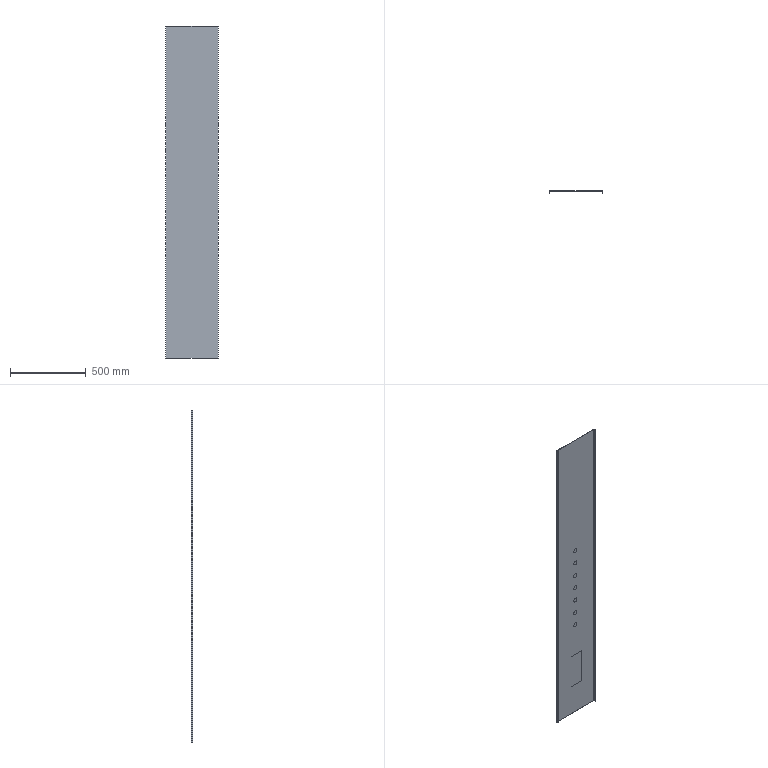Part | SolidWorks | features FlatPattern 1, ICE 1, SMBaseFlange 1, SheetMetal 1 | 1 solid | 48 faces | box 350 x 12 x 2194 mm | volume 1602003 mm3 | plane 30 | cylinder 18 | commonest cylinder face diameters 30 x14 0.4 x2 4.4 x2
STEP:
#1=CARTESIAN_POINT('',(0.,-0.5,685.));
#2=VERTEX_POINT('',#1);
#3=CARTESIAN_POINT('',(0.,-0.5,715.));
#4=VERTEX_POINT('',#3);
#5=CARTESIAN_POINT('',(0.,-0.5,700.));
#6=DIRECTION('',(0.,1.,0.));
#7=DIRECTION('',(0.,0.,1.));
#8=AXIS2_PLACEMENT_3D('',#5,#6,#7);
#9=CIRCLE('',#8,15.);
#10=EDGE_CURVE('',#2,#4,#9,.T.);
#11=ORIENTED_EDGE('',*,*,#10,.F.);
#12=CARTESIAN_POINT('',(0.,0.,685.));
#13=VERTEX_POINT('',#12);
#14=CARTESIAN_POINT('',(0.,-0.5,685.));
#15=DIRECTION('',(0.,1.,0.));
#16=VECTOR('',#15,1000.);
#17=LINE('',#14,#16);
#18=EDGE_CURVE('',#2,#13,#17,.T.);
#19=ORIENTED_EDGE('',*,*,#18,.T.);
#20=CARTESIAN_POINT('',(0.,0.,715.));
#21=VERTEX_POINT('',#20);
#22=CARTESIAN_POINT('',(0.,0.,700.));
#23=DIRECTION('',(0.,1.,0.));
#24=DIRECTION('',(0.,0.,1.));
#25=AXIS2_PLACEMENT_3D('',#22,#23,#24);
#26=CIRCLE('',#25,15.);
#27=EDGE_CURVE('',#13,#21,#26,.T.);
#28=ORIENTED_EDGE('',*,*,#27,.T.);
#29=CARTESIAN_POINT('',(0.,-0.5,715.));
#30=DIRECTION('',(0.,1.,0.));
#31=VECTOR('',#30,1000.);
#32=LINE('',#29,#31);
#33=EDGE_CURVE('',#4,#21,#32,.T.);
#34=ORIENTED_EDGE('',*,*,#33,.F.);
#35=EDGE_LOOP('',(#11,#19,#28,#34));
#36=FACE_OUTER_BOUND('',#35,.T.);
#37=CARTESIAN_POINT('',(0.,-0.5,700.));
#38=DIRECTION('',(0.,1.,0.));
#39=DIRECTION('',(0.,0.,1.));
#40=AXIS2_PLACEMENT_3D('',#37,#38,#39);
#41=CYLINDRICAL_SURFACE('',#40,15.);
#42=ADVANCED_FACE('',(#36),#41,.F.);
#43=CARTESIAN_POINT('',(0.,-0.5,785.));
#44=VERTEX_POINT('',#43);
#45=CARTESIAN_POINT('',(0.,-0.5,815.));
#46=VERTEX_POINT('',#45);
#47=CARTESIAN_POINT('',(0.,-0.5,800.));
#48=DIRECTION('',(0.,1.,0.));
#49=DIRECTION('',(0.,0.,1.));
#50=AXIS2_PLACEMENT_3D('',#47,#48,#49);
#51=CIRCLE('',#50,15.);
#52=EDGE_CURVE('',#44,#46,#51,.T.);
#53=ORIENTED_EDGE('',*,*,#52,.F.);
#54=CARTESIAN_POINT('',(0.,0.,785.));
#55=VERTEX_POINT('',#54);
#56=CARTESIAN_POINT('',(0.,-0.5,785.));
#57=DIRECTION('',(0.,1.,0.));
#58=VECTOR('',#57,1000.);
#59=LINE('',#56,#58);
#60=EDGE_CURVE('',#44,#55,#59,.T.);
#61=ORIENTED_EDGE('',*,*,#60,.T.);
#62=CARTESIAN_POINT('',(0.,0.,815.));
#63=VERTEX_POINT('',#62);
#64=CARTESIAN_POINT('',(0.,0.,800.));
#65=DIRECTION('',(0.,1.,0.));
#66=DIRECTION('',(0.,0.,1.));
#67=AXIS2_PLACEMENT_3D('',#64,#65,#66);
#68=CIRCLE('',#67,15.);
#69=EDGE_CURVE('',#55,#63,#68,.T.);
#70=ORIENTED_EDGE('',*,*,#69,.T.);
#71=CARTESIAN_POINT('',(0.,-0.5,815.));
#72=DIRECTION('',(0.,1.,0.));
#73=VECTOR('',#72,1000.);
#74=LINE('',#71,#73);
#75=EDGE_CURVE('',#46,#63,#74,.T.);
#76=ORIENTED_EDGE('',*,*,#75,.F.);
#77=EDGE_LOOP('',(#53,#61,#70,#76));
#78=FACE_OUTER_BOUND('',#77,.T.);
#79=CARTESIAN_POINT('',(0.,-0.5,800.));
#80=DIRECTION('',(0.,1.,0.));
#81=DIRECTION('',(0.,0.,1.));
#82=AXIS2_PLACEMENT_3D('',#79,#80,#81);
#83=CYLINDRICAL_SURFACE('',#82,15.);
#84=ADVANCED_FACE('',(#78),#83,.F.);
#85=CARTESIAN_POINT('',(0.,-0.5,885.));
#86=VERTEX_POINT('',#85);
#87=CARTESIAN_POINT('',(0.,-0.5,915.));
#88=VERTEX_POINT('',#87);
#89=CARTESIAN_POINT('',(0.,-0.5,900.));
#90=DIRECTION('',(0.,1.,0.));
#91=DIRECTION('',(0.,0.,1.));
#92=AXIS2_PLACEMENT_3D('',#89,#90,#91);
#93=CIRCLE('',#92,15.);
#94=EDGE_CURVE('',#86,#88,#93,.T.);
#95=ORIENTED_EDGE('',*,*,#94,.F.);
#96=CARTESIAN_POINT('',(0.,0.,885.));
#97=VERTEX_POINT('',#96);
#98=CARTESIAN_POINT('',(0.,-0.5,885.));
#99=DIRECTION('',(0.,1.,0.));
#100=VECTOR('',#99,1000.);
#101=LINE('',#98,#100);
#102=EDGE_CURVE('',#86,#97,#101,.T.);
#103=ORIENTED_EDGE('',*,*,#102,.T.);
#104=CARTESIAN_POINT('',(0.,0.,915.));
#105=VERTEX_POINT('',#104);
#106=CARTESIAN_POINT('',(0.,0.,900.));
#107=DIRECTION('',(0.,1.,0.));
#108=DIRECTION('',(0.,0.,1.));
#109=AXIS2_PLACEMENT_3D('',#106,#107,#108);
#110=CIRCLE('',#109,15.);
#111=EDGE_CURVE('',#97,#105,#110,.T.);
#112=ORIENTED_EDGE('',*,*,#111,.T.);
#113=CARTESIAN_POINT('',(0.,-0.5,915.));
#114=DIRECTION('',(0.,1.,0.));
#115=VECTOR('',#114,1000.);
#116=LINE('',#113,#115);
#117=EDGE_CURVE('',#88,#105,#116,.T.);
#118=ORIENTED_EDGE('',*,*,#117,.F.);
#119=EDGE_LOOP('',(#95,#103,#112,#118));
#120=FACE_OUTER_BOUND('',#119,.T.);
#121=CARTESIAN_POINT('',(0.,-0.5,900.));
#122=DIRECTION('',(0.,1.,0.));
#123=DIRECTION('',(0.,0.,1.));
#124=AXIS2_PLACEMENT_3D('',#121,#122,#123);
#125=CYLINDRICAL_SURFACE('',#124,15.);
#126=ADVANCED_FACE('',(#120),#125,.F.);
#127=CARTESIAN_POINT('',(0.,-0.5,985.));
#128=VERTEX_POINT('',#127);
#129=CARTESIAN_POINT('',(0.,-0.5,1015.));
#130=VERTEX_POINT('',#129);
#131=CARTESIAN_POINT('',(0.,-0.5,1000.));
#132=DIRECTION('',(0.,1.,0.));
#133=DIRECTION('',(0.,0.,1.));
#134=AXIS2_PLACEMENT_3D('',#131,#132,#133);
#135=CIRCLE('',#134,15.);
#136=EDGE_CURVE('',#128,#130,#135,.T.);
#137=ORIENTED_EDGE('',*,*,#136,.F.);
#138=CARTESIAN_POINT('',(0.,0.,985.));
#139=VERTEX_POINT('',#138);
#140=CARTESIAN_POINT('',(0.,-0.5,985.));
#141=DIRECTION('',(0.,1.,0.));
#142=VECTOR('',#141,1000.);
#143=LINE('',#140,#142);
#144=EDGE_CURVE('',#128,#139,#143,.T.);
#145=ORIENTED_EDGE('',*,*,#144,.T.);
#146=CARTESIAN_POINT('',(0.,0.,1015.));
#147=VERTEX_POINT('',#146);
#148=CARTESIAN_POINT('',(0.,0.,1000.));
#149=DIRECTION('',(0.,1.,0.));
#150=DIRECTION('',(0.,0.,1.));
#151=AXIS2_PLACEMENT_3D('',#148,#149,#150);
#152=CIRCLE('',#151,15.);
#153=EDGE_CURVE('',#139,#147,#152,.T.);
#154=ORIENTED_EDGE('',*,*,#153,.T.);
#155=CARTESIAN_POINT('',(0.,-0.5,1015.));
#156=DIRECTION('',(0.,1.,0.));
#157=VECTOR('',#156,1000.);
#158=LINE('',#155,#157);
#159=EDGE_CURVE('',#130,#147,#158,.T.);
#160=ORIENTED_EDGE('',*,*,#159,.F.);
#161=EDGE_LOOP('',(#137,#145,#154,#160));
#162=FACE_OUTER_BOUND('',#161,.T.);
#163=CARTESIAN_POINT('',(0.,-0.5,1000.));
#164=DIRECTION('',(0.,1.,0.));
#165=DIRECTION('',(0.,0.,1.));
#166=AXIS2_PLACEMENT_3D('',#163,#164,#165);
#167=CYLINDRICAL_SURFACE('',#166,15.);
#168=ADVANCED_FACE('',(#162),#167,.F.);
#169=CARTESIAN_POINT('',(0.,-0.5,1085.));
#170=VERTEX_POINT('',#169);
#171=CARTESIAN_POINT('',(0.,-0.5,1115.));
#172=VERTEX_POINT('',#171);
#173=CARTESIAN_POINT('',(0.,-0.5,1100.));
#174=DIRECTION('',(0.,1.,0.));
#175=DIRECTION('',(0.,0.,1.));
#176=AXIS2_PLACEMENT_3D('',#173,#174,#175);
#177=CIRCLE('',#176,15.);
#178=EDGE_CURVE('',#170,#172,#177,.T.);
#179=ORIENTED_EDGE('',*,*,#178,.F.);
#180=CARTESIAN_POINT('',(0.,0.,1085.));
#181=VERTEX_POINT('',#180);
#182=CARTESIAN_POINT('',(0.,-0.5,1085.));
#183=DIRECTION('',(0.,1.,0.));
#184=VECTOR('',#183,1000.);
#185=LINE('',#182,#184);
#186=EDGE_CURVE('',#170,#181,#185,.T.);
#187=ORIENTED_EDGE('',*,*,#186,.T.);
#188=CARTESIAN_POINT('',(0.,0.,1115.));
#189=VERTEX_POINT('',#188);
#190=CARTESIAN_POINT('',(0.,0.,1100.));
#191=DIRECTION('',(0.,1.,0.));
#192=DIRECTION('',(0.,0.,1.));
#193=AXIS2_PLACEMENT_3D('',#190,#191,#192);
#194=CIRCLE('',#193,15.);
#195=EDGE_CURVE('',#181,#189,#194,.T.);
#196=ORIENTED_EDGE('',*,*,#195,.T.);
#197=CARTESIAN_POINT('',(0.,-0.5,1115.));
#198=DIRECTION('',(0.,1.,0.));
#199=VECTOR('',#198,1000.);
#200=LINE('',#197,#199);
#201=EDGE_CURVE('',#172,#189,#200,.T.);
#202=ORIENTED_EDGE('',*,*,#201,.F.);
#203=EDGE_LOOP('',(#179,#187,#196,#202));
#204=FACE_OUTER_BOUND('',#203,.T.);
#205=CARTESIAN_POINT('',(0.,-0.5,1100.));
#206=DIRECTION('',(0.,1.,0.));
#207=DIRECTION('',(0.,0.,1.));
#208=AXIS2_PLACEMENT_3D('',#205,#206,#207);
#209=CYLINDRICAL_SURFACE('',#208,15.);
#210=ADVANCED_FACE('',(#204),#209,.F.);
#211=CARTESIAN_POINT('',(0.,-0.5,1185.));
#212=VERTEX_POINT('',#211);
#213=CARTESIAN_POINT('',(0.,-0.5,1215.));
#214=VERTEX_POINT('',#213);
#215=CARTESIAN_POINT('',(0.,-0.5,1200.));
#216=DIRECTION('',(0.,1.,0.));
#217=DIRECTION('',(0.,0.,1.));
#218=AXIS2_PLACEMENT_3D('',#215,#216,#217);
#219=CIRCLE('',#218,15.);
#220=EDGE_CURVE('',#212,#214,#219,.T.);
#221=ORIENTED_EDGE('',*,*,#220,.F.);
#222=CARTESIAN_POINT('',(0.,0.,1185.));
#223=VERTEX_POINT('',#222);
#224=CARTESIAN_POINT('',(0.,-0.5,1185.));
#225=DIRECTION('',(0.,1.,0.));
#226=VECTOR('',#225,1000.);
#227=LINE('',#224,#226);
#228=EDGE_CURVE('',#212,#223,#227,.T.);
#229=ORIENTED_EDGE('',*,*,#228,.T.);
#230=CARTESIAN_POINT('',(0.,0.,1215.));
#231=VERTEX_POINT('',#230);
#232=CARTESIAN_POINT('',(0.,0.,1200.));
#233=DIRECTION('',(0.,1.,0.));
#234=DIRECTION('',(0.,0.,1.));
#235=AXIS2_PLACEMENT_3D('',#232,#233,#234);
#236=CIRCLE('',#235,15.);
#237=EDGE_CURVE('',#223,#231,#236,.T.);
#238=ORIENTED_EDGE('',*,*,#237,.T.);
#239=CARTESIAN_POINT('',(0.,-0.5,1215.));
#240=DIRECTION('',(0.,1.,0.));
#241=VECTOR('',#240,1000.);
#242=LINE('',#239,#241);
#243=EDGE_CURVE('',#214,#231,#242,.T.);
#244=ORIENTED_EDGE('',*,*,#243,.F.);
#245=EDGE_LOOP('',(#221,#229,#238,#244));
#246=FACE_OUTER_BOUND('',#245,.T.);
#247=CARTESIAN_POINT('',(0.,-0.5,1200.));
#248=DIRECTION('',(0.,1.,0.));
#249=DIRECTION('',(0.,0.,1.));
#250=AXIS2_PLACEMENT_3D('',#247,#248,#249);
#251=CYLINDRICAL_SURFACE('',#250,15.);
#252=ADVANCED_FACE('',(#246),#251,.F.);
#253=CARTESIAN_POINT('',(0.,-0.5,1285.));
#254=VERTEX_POINT('',#253);
#255=CARTESIAN_POINT('',(0.,-0.5,1315.));
#256=VERTEX_POINT('',#255);
#257=CARTESIAN_POINT('',(0.,-0.5,1300.));
#258=DIRECTION('',(0.,1.,0.));
#259=DIRECTION('',(0.,0.,1.));
#260=AXIS2_PLACEMENT_3D('',#257,#258,#259);
#261=CIRCLE('',#260,15.);
#262=EDGE_CURVE('',#254,#256,#261,.T.);
#263=ORIENTED_EDGE('',*,*,#262,.F.);
#264=CARTESIAN_POINT('',(0.,0.,1285.));
#265=VERTEX_POINT('',#264);
#266=CARTESIAN_POINT('',(0.,-0.5,1285.));
#267=DIRECTION('',(0.,1.,0.));
#268=VECTOR('',#267,1000.);
#269=LINE('',#266,#268);
#270=EDGE_CURVE('',#254,#265,#269,.T.);
#271=ORIENTED_EDGE('',*,*,#270,.T.);
#272=CARTESIAN_POINT('',(0.,0.,1315.));
#273=VERTEX_POINT('',#272);
#274=CARTESIAN_POINT('',(0.,0.,1300.));
#275=DIRECTION('',(0.,1.,0.));
#276=DIRECTION('',(0.,0.,1.));
#277=AXIS2_PLACEMENT_3D('',#274,#275,#276);
#278=CIRCLE('',#277,15.);
#279=EDGE_CURVE('',#265,#273,#278,.T.);
#280=ORIENTED_EDGE('',*,*,#279,.T.);
#281=CARTESIAN_POINT('',(0.,-0.5,1315.));
#282=DIRECTION('',(0.,1.,0.));
#283=VECTOR('',#282,1000.);
#284=LINE('',#281,#283);
#285=EDGE_CURVE('',#256,#273,#284,.T.);
#286=ORIENTED_EDGE('',*,*,#285,.F.);
#287=EDGE_LOOP('',(#263,#271,#280,#286));
#288=FACE_OUTER_BOUND('',#287,.T.);
#289=CARTESIAN_POINT('',(0.,-0.5,1300.));
#290=DIRECTION('',(0.,1.,0.));
#291=DIRECTION('',(0.,0.,1.));
#292=AXIS2_PLACEMENT_3D('',#289,#290,#291);
#293=CYLINDRICAL_SURFACE('',#292,15.);
#294=ADVANCED_FACE('',(#288),#293,.F.);
#295=CARTESIAN_POINT('',(-172.8,0.,2194.));
#296=VERTEX_POINT('',#295);
#297=CARTESIAN_POINT('',(-172.8,-2.,2194.));
#298=VERTEX_POINT('',#297);
#299=CARTESIAN_POINT('',(-172.8,0.,2194.));
#300=DIRECTION('',(0.,-1.,0.));
#301=VECTOR('',#300,1000.);
#302=LINE('',#299,#301);
#303=EDGE_CURVE('',#296,#298,#302,.T.);
#304=ORIENTED_EDGE('',*,*,#303,.F.);
#305=CARTESIAN_POINT('',(-175.,-2.2,2194.));
#306=VERTEX_POINT('',#305);
#307=CARTESIAN_POINT('',(-172.8,-2.2,2194.));
#308=DIRECTION('',(0.,0.,-1.));
#309=DIRECTION('',(1.,0.,0.));
#310=AXIS2_PLACEMENT_3D('',#307,#308,#309);
#311=CIRCLE('',#310,2.2);
#312=EDGE_CURVE('',#306,#296,#311,.T.);
#313=ORIENTED_EDGE('',*,*,#312,.F.);
#314=CARTESIAN_POINT('',(-173.,-2.2,2194.));
#315=VERTEX_POINT('',#314);
#316=CARTESIAN_POINT('',(-173.,-2.2,2194.));
#317=DIRECTION('',(-1.,0.,0.));
#318=VECTOR('',#317,1000.);
#319=LINE('',#316,#318);
#320=EDGE_CURVE('',#315,#306,#319,.T.);
#321=ORIENTED_EDGE('',*,*,#320,.F.);
#322=CARTESIAN_POINT('',(-172.8,-2.2,2194.));
#323=DIRECTION('',(0.,0.,-1.));
#324=DIRECTION('',(1.,0.,0.));
#325=AXIS2_PLACEMENT_3D('',#322,#323,#324);
#326=CIRCLE('',#325,0.2);
#327=EDGE_CURVE('',#315,#298,#326,.T.);
#328=ORIENTED_EDGE('',*,*,#327,.T.);
#329=EDGE_LOOP('',(#304,#313,#321,#328));
#330=FACE_OUTER_BOUND('',#329,.T.);
#331=CARTESIAN_POINT('',(-172.8,0.,2194.));
#332=DIRECTION('',(0.,0.,1.));
#333=DIRECTION('',(1.,0.,0.));
#334=AXIS2_PLACEMENT_3D('',#331,#332,#333);
#335=PLANE('',#334);
#336=ADVANCED_FACE('',(#330),#335,.T.);
#337=CARTESIAN_POINT('',(172.8,0.,2194.));
#338=VERTEX_POINT('',#337);
#339=CARTESIAN_POINT('',(-175.,0.,2194.));
#340=DIRECTION('',(1.,0.,0.));
#341=VECTOR('',#340,1000.);
#342=LINE('',#339,#341);
#343=EDGE_CURVE('',#296,#338,#342,.T.);
#344=ORIENTED_EDGE('',*,*,#343,.F.);
#345=ORIENTED_EDGE('',*,*,#303,.T.);
#346=CARTESIAN_POINT('',(172.8,-2.,2194.));
#347=VERTEX_POINT('',#346);
#348=CARTESIAN_POINT('',(-175.,-2.,2194.));
#349=DIRECTION('',(1.,0.,0.));
#350=VECTOR('',#349,1000.);
#351=LINE('',#348,#350);
#352=EDGE_CURVE('',#298,#347,#351,.T.);
#353=ORIENTED_EDGE('',*,*,#352,.T.);
#354=CARTESIAN_POINT('',(172.8,-2.,2194.));
#355=DIRECTION('',(0.,1.,0.));
#356=VECTOR('',#355,1000.);
#357=LINE('',#354,#356);
#358=EDGE_CURVE('',#347,#338,#357,.T.);
#359=ORIENTED_EDGE('',*,*,#358,.T.);
#360=EDGE_LOOP('',(#344,#345,#353,#359));
#361=FACE_OUTER_BOUND('',#360,.T.);
#362=CARTESIAN_POINT('',(-173.,-2.2,2194.));
#363=DIRECTION('',(0.,0.,1.));
#364=DIRECTION('',(1.,0.,0.));
#365=AXIS2_PLACEMENT_3D('',#362,#363,#364);
#366=PLANE('',#365);
#367=ADVANCED_FACE('',(#361),#366,.T.);
#368=CARTESIAN_POINT('',(-175.,-2.2,0.));
#369=VERTEX_POINT('',#368);
#370=CARTESIAN_POINT('',(-173.,-2.2,0.));
#371=VERTEX_POINT('',#370);
#372=CARTESIAN_POINT('',(-175.,-2.2,0.));
#373=DIRECTION('',(1.,0.,0.));
#374=VECTOR('',#373,1000.);
#375=LINE('',#372,#374);
#376=EDGE_CURVE('',#369,#371,#375,.T.);
#377=ORIENTED_EDGE('',*,*,#376,.F.);
#378=CARTESIAN_POINT('',(-172.8,0.,0.));
#379=VERTEX_POINT('',#378);
#380=CARTESIAN_POINT('',(-172.8,-2.2,0.));
#381=DIRECTION('',(0.,0.,-1.));
#382=DIRECTION('',(1.,0.,0.));
#383=AXIS2_PLACEMENT_3D('',#380,#381,#382);
#384=CIRCLE('',#383,2.2);
#385=EDGE_CURVE('',#369,#379,#384,.T.);
#386=ORIENTED_EDGE('',*,*,#385,.T.);
#387=CARTESIAN_POINT('',(-172.8,-2.,0.));
#388=VERTEX_POINT('',#387);
#389=CARTESIAN_POINT('',(-172.8,-2.,0.));
#390=DIRECTION('',(0.,1.,0.));
#391=VECTOR('',#390,1000.);
#392=LINE('',#389,#391);
#393=EDGE_CURVE('',#388,#379,#392,.T.);
#394=ORIENTED_EDGE('',*,*,#393,.F.);
#395=CARTESIAN_POINT('',(-172.8,-2.2,0.));
#396=DIRECTION('',(0.,0.,-1.));
#397=DIRECTION('',(1.,0.,0.));
#398=AXIS2_PLACEMENT_3D('',#395,#396,#397);
#399=CIRCLE('',#398,0.2);
#400=EDGE_CURVE('',#371,#388,#399,.T.);
#401=ORIENTED_EDGE('',*,*,#400,.F.);
#402=EDGE_LOOP('',(#377,#386,#394,#401));
#403=FACE_OUTER_BOUND('',#402,.T.);
#404=CARTESIAN_POINT('',(-175.,-2.2,0.));
#405=DIRECTION('',(0.,0.,-1.));
#406=DIRECTION('',(-1.,0.,0.));
#407=AXIS2_PLACEMENT_3D('',#404,#405,#406);
#408=PLANE('',#407);
#409=ADVANCED_FACE('',(#403),#408,.T.);
#410=CARTESIAN_POINT('',(-175.,-12.,0.));
#411=VERTEX_POINT('',#410);
#412=CARTESIAN_POINT('',(-175.,-12.,0.));
#413=DIRECTION('',(0.,1.,0.));
#414=VECTOR('',#413,1000.);
#415=LINE('',#412,#414);
#416=EDGE_CURVE('',#411,#369,#415,.T.);
#417=ORIENTED_EDGE('',*,*,#416,.T.);
#418=ORIENTED_EDGE('',*,*,#376,.T.);
#419=CARTESIAN_POINT('',(-173.,-12.,0.));
#420=VERTEX_POINT('',#419);
#421=CARTESIAN_POINT('',(-173.,-12.,0.));
#422=DIRECTION('',(0.,1.,0.));
#423=VECTOR('',#422,1000.);
#424=LINE('',#421,#423);
#425=EDGE_CURVE('',#420,#371,#424,.T.);
#426=ORIENTED_EDGE('',*,*,#425,.F.);
#427=CARTESIAN_POINT('',(-173.,-12.,0.));
#428=DIRECTION('',(-1.,0.,0.));
#429=VECTOR('',#428,1000.);
#430=LINE('',#427,#429);
#431=EDGE_CURVE('',#420,#411,#430,.T.);
#432=ORIENTED_EDGE('',*,*,#431,.T.);
#433=EDGE_LOOP('',(#417,#418,#426,#432));
#434=FACE_OUTER_BOUND('',#433,.T.);
#435=CARTESIAN_POINT('',(-172.8,-2.,0.));
#436=DIRECTION('',(0.,0.,-1.));
#437=DIRECTION('',(-1.,0.,0.));
#438=AXIS2_PLACEMENT_3D('',#435,#436,#437);
#439=PLANE('',#438);
#440=ADVANCED_FACE('',(#434),#439,.T.);
#441=CARTESIAN_POINT('',(175.,-2.2,2194.));
#442=VERTEX_POINT('',#441);
#443=CARTESIAN_POINT('',(173.,-2.2,2194.));
#444=VERTEX_POINT('',#443);
#445=CARTESIAN_POINT('',(175.,-2.2,2194.));
#446=DIRECTION('',(-1.,0.,0.));
#447=VECTOR('',#446,1000.);
#448=LINE('',#445,#447);
#449=EDGE_CURVE('',#442,#444,#448,.T.);
#450=ORIENTED_EDGE('',*,*,#449,.F.);
#451=CARTESIAN_POINT('',(172.8,-2.2,2194.));
#452=DIRECTION('',(0.,0.,-1.));
#453=DIRECTION('',(1.,0.,0.));
#454=AXIS2_PLACEMENT_3D('',#451,#452,#453);
#455=CIRCLE('',#454,2.2);
#456=EDGE_CURVE('',#338,#442,#455,.T.);
#457=ORIENTED_EDGE('',*,*,#456,.F.);
#458=ORIENTED_EDGE('',*,*,#358,.F.);
#459=CARTESIAN_POINT('',(172.8,-2.2,2194.));
#460=DIRECTION('',(0.,0.,-1.));
#461=DIRECTION('',(1.,0.,0.));
#462=AXIS2_PLACEMENT_3D('',#459,#460,#461);
#463=CIRCLE('',#462,0.2);
#464=EDGE_CURVE('',#347,#444,#463,.T.);
#465=ORIENTED_EDGE('',*,*,#464,.T.);
#466=EDGE_LOOP('',(#450,#457,#458,#465));
#467=FACE_OUTER_BOUND('',#466,.T.);
#468=CARTESIAN_POINT('',(175.,-2.2,2194.));
#469=DIRECTION('',(0.,0.,1.));
#470=DIRECTION('',(1.,0.,0.));
#471=AXIS2_PLACEMENT_3D('',#468,#469,#470);
#472=PLANE('',#471);
#473=ADVANCED_FACE('',(#467),#472,.T.);
#474=CARTESIAN_POINT('',(175.,-12.,2194.));
#475=VERTEX_POINT('',#474);
#476=CARTESIAN_POINT('',(175.,0.,2194.));
#477=DIRECTION('',(0.,-1.,0.));
#478=VECTOR('',#477,1000.);
#479=LINE('',#476,#478);
#480=EDGE_CURVE('',#442,#475,#479,.T.);
#481=ORIENTED_EDGE('',*,*,#480,.F.);
#482=ORIENTED_EDGE('',*,*,#449,.T.);
#483=CARTESIAN_POINT('',(173.,-12.,2194.));
#484=VERTEX_POINT('',#483);
#485=CARTESIAN_POINT('',(173.,0.,2194.));
#486=DIRECTION('',(0.,-1.,0.));
#487=VECTOR('',#486,1000.);
#488=LINE('',#485,#487);
#489=EDGE_CURVE('',#444,#484,#488,.T.);
#490=ORIENTED_EDGE('',*,*,#489,.T.);
#491=CARTESIAN_POINT('',(175.,-12.,2194.));
#492=DIRECTION('',(-1.,0.,0.));
#493=VECTOR('',#492,1000.);
#494=LINE('',#491,#493);
#495=EDGE_CURVE('',#475,#484,#494,.T.);
#496=ORIENTED_EDGE('',*,*,#495,.F.);
#497=EDGE_LOOP('',(#481,#482,#490,#496));
#498=FACE_OUTER_BOUND('',#497,.T.);
#499=CARTESIAN_POINT('',(172.8,-2.,2194.));
#500=DIRECTION('',(0.,0.,1.));
#501=DIRECTION('',(1.,0.,0.));
#502=AXIS2_PLACEMENT_3D('',#499,#500,#501);
#503=PLANE('',#502);
#504=ADVANCED_FACE('',(#498),#503,.T.);
#505=CARTESIAN_POINT('',(172.8,0.,0.));
#506=VERTEX_POINT('',#505);
#507=CARTESIAN_POINT('',(172.8,-2.,0.));
#508=VERTEX_POINT('',#507);
#509=CARTESIAN_POINT('',(172.8,0.,0.));
#510=DIRECTION('',(0.,-1.,0.));
#511=VECTOR('',#510,1000.);
#512=LINE('',#509,#511);
#513=EDGE_CURVE('',#506,#508,#512,.T.);
#514=ORIENTED_EDGE('',*,*,#513,.F.);
#515=CARTESIAN_POINT('',(175.,-2.2,0.));
#516=VERTEX_POINT('',#515);
#517=CARTESIAN_POINT('',(172.8,-2.2,0.));
#518=DIRECTION('',(0.,0.,-1.));
#519=DIRECTION('',(1.,0.,0.));
#520=AXIS2_PLACEMENT_3D('',#517,#518,#519);
#521=CIRCLE('',#520,2.2);
#522=EDGE_CURVE('',#506,#516,#521,.T.);
#523=ORIENTED_EDGE('',*,*,#522,.T.);
#524=CARTESIAN_POINT('',(173.,-2.2,0.));
#525=VERTEX_POINT('',#524);
#526=CARTESIAN_POINT('',(173.,-2.2,0.));
#527=DIRECTION('',(1.,0.,0.));
#528=VECTOR('',#527,1000.);
#529=LINE('',#526,#528);
#530=EDGE_CURVE('',#525,#516,#529,.T.);
#531=ORIENTED_EDGE('',*,*,#530,.F.);
#532=CARTESIAN_POINT('',(172.8,-2.2,0.));
#533=DIRECTION('',(0.,0.,-1.));
#534=DIRECTION('',(1.,0.,0.));
#535=AXIS2_PLACEMENT_3D('',#532,#533,#534);
#536=CIRCLE('',#535,0.2);
#537=EDGE_CURVE('',#508,#525,#536,.T.);
#538=ORIENTED_EDGE('',*,*,#537,.F.);
#539=EDGE_LOOP('',(#514,#523,#531,#538));
#540=FACE_OUTER_BOUND('',#539,.T.);
#541=CARTESIAN_POINT('',(172.8,0.,0.));
#542=DIRECTION('',(0.,0.,-1.));
#543=DIRECTION('',(-1.,0.,0.));
#544=AXIS2_PLACEMENT_3D('',#541,#542,#543);
#545=PLANE('',#544);
#546=ADVANCED_FACE('',(#540),#545,.T.);
#547=CARTESIAN_POINT('',(-175.,0.,0.));
#548=DIRECTION('',(1.,0.,0.));
#549=VECTOR('',#548,1000.);
#550=LINE('',#547,#549);
#551=EDGE_CURVE('',#379,#506,#550,.T.);
#552=ORIENTED_EDGE('',*,*,#551,.T.);
#553=ORIENTED_EDGE('',*,*,#513,.T.);
#554=CARTESIAN_POINT('',(-175.,-2.,0.));
#555=DIRECTION('',(1.,0.,0.));
#556=VECTOR('',#555,1000.);
#557=LINE('',#554,#556);
#558=EDGE_CURVE('',#388,#508,#557,.T.);
#559=ORIENTED_EDGE('',*,*,#558,.F.);
#560=ORIENTED_EDGE('',*,*,#393,.T.);
#561=EDGE_LOOP('',(#552,#553,#559,#560));
#562=FACE_OUTER_BOUND('',#561,.T.);
#563=CARTESIAN_POINT('',(173.,-2.2,0.));
#564=DIRECTION('',(0.,0.,-1.));
#565=DIRECTION('',(-1.,0.,0.));
#566=AXIS2_PLACEMENT_3D('',#563,#564,#565);
#567=PLANE('',#566);
#568=ADVANCED_FACE('',(#562),#567,.T.);
#569=CARTESIAN_POINT('',(173.,-12.,0.));
#570=VERTEX_POINT('',#569);
#571=CARTESIAN_POINT('',(173.,0.,0.));
#572=DIRECTION('',(0.,-1.,0.));
#573=VECTOR('',#572,1000.);
#574=LINE('',#571,#573);
#575=EDGE_CURVE('',#525,#570,#574,.T.);
#576=ORIENTED_EDGE('',*,*,#575,.T.);
#577=CARTESIAN_POINT('',(173.,-12.,2194.));
#578=DIRECTION('',(0.,0.,-1.));
#579=VECTOR('',#578,1000.);
#580=LINE('',#577,#579);
#581=EDGE_CURVE('',#484,#570,#580,.T.);
#582=ORIENTED_EDGE('',*,*,#581,.F.);
#583=ORIENTED_EDGE('',*,*,#489,.F.);
#584=CARTESIAN_POINT('',(173.,-2.2,2194.));
#585=DIRECTION('',(0.,0.,-1.));
#586=VECTOR('',#585,1000.);
#587=LINE('',#584,#586);
#588=EDGE_CURVE('',#444,#525,#587,.T.);
#589=ORIENTED_EDGE('',*,*,#588,.T.);
#590=EDGE_LOOP('',(#576,#582,#583,#589));
#591=FACE_OUTER_BOUND('',#590,.T.);
#592=CARTESIAN_POINT('',(173.,0.,2194.));
#593=DIRECTION('',(1.,0.,0.));
#594=DIRECTION('',(0.,0.,-1.));
#595=AXIS2_PLACEMENT_3D('',#592,#593,#594);
#596=PLANE('',#595);
#597=ADVANCED_FACE('',(#591),#596,.F.);
#598=CARTESIAN_POINT('',(175.,-12.,0.));
#599=VERTEX_POINT('',#598);
#600=CARTESIAN_POINT('',(175.,-12.,0.));
#601=DIRECTION('',(-1.,0.,0.));
#602=VECTOR('',#601,1000.);
#603=LINE('',#600,#602);
#604=EDGE_CURVE('',#599,#570,#603,.T.);
#605=ORIENTED_EDGE('',*,*,#604,.F.);
#606=CARTESIAN_POINT('',(175.,-12.,2194.));
#607=DIRECTION('',(0.,0.,-1.));
#608=VECTOR('',#607,1000.);
#609=LINE('',#606,#608);
#610=EDGE_CURVE('',#475,#599,#609,.T.);
#611=ORIENTED_EDGE('',*,*,#610,.F.);
#612=ORIENTED_EDGE('',*,*,#495,.T.);
#613=ORIENTED_EDGE('',*,*,#581,.T.);
#614=EDGE_LOOP('',(#605,#611,#612,#613));
#615=FACE_OUTER_BOUND('',#614,.T.);
#616=CARTESIAN_POINT('',(175.,-12.,2194.));
#617=DIRECTION('',(0.,-1.,0.));
#618=DIRECTION('',(0.,0.,-1.));
#619=AXIS2_PLACEMENT_3D('',#616,#617,#618);
#620=PLANE('',#619);
#621=ADVANCED_FACE('',(#615),#620,.T.);
#622=CARTESIAN_POINT('',(175.,0.,0.));
#623=DIRECTION('',(0.,-1.,0.));
#624=VECTOR('',#623,1000.);
#625=LINE('',#622,#624);
#626=EDGE_CURVE('',#516,#599,#625,.T.);
#627=ORIENTED_EDGE('',*,*,#626,.F.);
#628=CARTESIAN_POINT('',(175.,-2.2,2194.));
#629=DIRECTION('',(0.,0.,-1.));
#630=VECTOR('',#629,1000.);
#631=LINE('',#628,#630);
#632=EDGE_CURVE('',#442,#516,#631,.T.);
#633=ORIENTED_EDGE('',*,*,#632,.F.);
#634=ORIENTED_EDGE('',*,*,#480,.T.);
#635=ORIENTED_EDGE('',*,*,#610,.T.);
#636=EDGE_LOOP('',(#627,#633,#634,#635));
#637=FACE_OUTER_BOUND('',#636,.T.);
#638=CARTESIAN_POINT('',(175.,0.,2194.));
#639=DIRECTION('',(1.,0.,0.));
#640=DIRECTION('',(0.,0.,-1.));
#641=AXIS2_PLACEMENT_3D('',#638,#639,#640);
#642=PLANE('',#641);
#643=ADVANCED_FACE('',(#637),#642,.T.);
#644=ORIENTED_EDGE('',*,*,#522,.F.);
#645=CARTESIAN_POINT('',(172.8,0.,2194.));
#646=DIRECTION('',(0.,0.,-1.));
#647=VECTOR('',#646,1000.);
#648=LINE('',#645,#647);
#649=EDGE_CURVE('',#338,#506,#648,.T.);
#650=ORIENTED_EDGE('',*,*,#649,.F.);
#651=ORIENTED_EDGE('',*,*,#456,.T.);
#652=ORIENTED_EDGE('',*,*,#632,.T.);
#653=EDGE_LOOP('',(#644,#650,#651,#652));
#654=FACE_OUTER_BOUND('',#653,.T.);
#655=CARTESIAN_POINT('',(172.8,-2.2,2194.));
#656=DIRECTION('',(0.,0.,-1.));
#657=DIRECTION('',(-1.,0.,0.));
#658=AXIS2_PLACEMENT_3D('',#655,#656,#657);
#659=CYLINDRICAL_SURFACE('',#658,2.2);
#660=ADVANCED_FACE('',(#654),#659,.T.);
#661=CARTESIAN_POINT('',(59.974,0.,460.46));
#662=VERTEX_POINT('',#661);
#663=CARTESIAN_POINT('',(59.974,0.,217.636));
#664=VERTEX_POINT('',#663);
#665=CARTESIAN_POINT('',(59.974,0.,217.636));
#666=DIRECTION('',(0.,0.,-1.));
#667=VECTOR('',#666,1000.);
#668=LINE('',#665,#667);
#669=EDGE_CURVE('',#662,#664,#668,.T.);
#670=ORIENTED_EDGE('',*,*,#669,.F.);
#671=CARTESIAN_POINT('',(-59.974,0.,460.46));
#672=VERTEX_POINT('',#671);
#673=CARTESIAN_POINT('',(-59.974,0.,460.46));
#674=DIRECTION('',(1.,0.,0.));
#675=VECTOR('',#674,1000.);
#676=LINE('',#673,#675);
#677=EDGE_CURVE('',#672,#662,#676,.T.);
#678=ORIENTED_EDGE('',*,*,#677,.F.);
#679=CARTESIAN_POINT('',(-59.974,0.,217.636));
#680=VERTEX_POINT('',#679);
#681=CARTESIAN_POINT('',(-59.974,0.,217.636));
#682=DIRECTION('',(0.,0.,1.));
#683=VECTOR('',#682,1000.);
#684=LINE('',#681,#683);
#685=EDGE_CURVE('',#680,#672,#684,.T.);
#686=ORIENTED_EDGE('',*,*,#685,.F.);
#687=CARTESIAN_POINT('',(-59.974,0.,217.636));
#688=DIRECTION('',(-1.,0.,0.));
#689=VECTOR('',#688,1000.);
#690=LINE('',#687,#689);
#691=EDGE_CURVE('',#664,#680,#690,.T.);
#692=ORIENTED_EDGE('',*,*,#691,.F.);
#693=EDGE_LOOP('',(#670,#678,#686,#692));
#694=FACE_BOUND('',#693,.T.);
#695=CARTESIAN_POINT('',(0.,0.,700.));
#696=DIRECTION('',(0.,1.,0.));
#697=DIRECTION('',(0.,0.,1.));
#698=AXIS2_PLACEMENT_3D('',#695,#696,#697);
#699=CIRCLE('',#698,15.);
#700=EDGE_CURVE('',#21,#13,#699,.T.);
#701=ORIENTED_EDGE('',*,*,#700,.F.);
#702=ORIENTED_EDGE('',*,*,#27,.F.);
#703=EDGE_LOOP('',(#701,#702));
#704=FACE_BOUND('',#703,.T.);
#705=CARTESIAN_POINT('',(0.,0.,800.));
#706=DIRECTION('',(0.,1.,0.));
#707=DIRECTION('',(0.,0.,1.));
#708=AXIS2_PLACEMENT_3D('',#705,#706,#707);
#709=CIRCLE('',#708,15.);
#710=EDGE_CURVE('',#63,#55,#709,.T.);
#711=ORIENTED_EDGE('',*,*,#710,.F.);
#712=ORIENTED_EDGE('',*,*,#69,.F.);
#713=EDGE_LOOP('',(#711,#712));
#714=FACE_BOUND('',#713,.T.);
#715=CARTESIAN_POINT('',(0.,0.,900.));
#716=DIRECTION('',(0.,1.,0.));
#717=DIRECTION('',(0.,0.,1.));
#718=AXIS2_PLACEMENT_3D('',#715,#716,#717);
#719=CIRCLE('',#718,15.);
#720=EDGE_CURVE('',#105,#97,#719,.T.);
#721=ORIENTED_EDGE('',*,*,#720,.F.);
#722=ORIENTED_EDGE('',*,*,#111,.F.);
#723=EDGE_LOOP('',(#721,#722));
#724=FACE_BOUND('',#723,.T.);
#725=CARTESIAN_POINT('',(0.,0.,1000.));
#726=DIRECTION('',(0.,1.,0.));
#727=DIRECTION('',(0.,0.,1.));
#728=AXIS2_PLACEMENT_3D('',#725,#726,#727);
#729=CIRCLE('',#728,15.);
#730=EDGE_CURVE('',#147,#139,#729,.T.);
#731=ORIENTED_EDGE('',*,*,#730,.F.);
#732=ORIENTED_EDGE('',*,*,#153,.F.);
#733=EDGE_LOOP('',(#731,#732));
#734=FACE_BOUND('',#733,.T.);
#735=CARTESIAN_POINT('',(0.,0.,1100.));
#736=DIRECTION('',(0.,1.,0.));
#737=DIRECTION('',(0.,0.,1.));
#738=AXIS2_PLACEMENT_3D('',#735,#736,#737);
#739=CIRCLE('',#738,15.);
#740=EDGE_CURVE('',#189,#181,#739,.T.);
#741=ORIENTED_EDGE('',*,*,#740,.F.);
#742=ORIENTED_EDGE('',*,*,#195,.F.);
#743=EDGE_LOOP('',(#741,#742));
#744=FACE_BOUND('',#743,.T.);
#745=CARTESIAN_POINT('',(0.,0.,1200.));
#746=DIRECTION('',(0.,1.,0.));
#747=DIRECTION('',(0.,0.,1.));
#748=AXIS2_PLACEMENT_3D('',#745,#746,#747);
#749=CIRCLE('',#748,15.);
#750=EDGE_CURVE('',#231,#223,#749,.T.);
#751=ORIENTED_EDGE('',*,*,#750,.F.);
#752=ORIENTED_EDGE('',*,*,#237,.F.);
#753=EDGE_LOOP('',(#751,#752));
#754=FACE_BOUND('',#753,.T.);
#755=CARTESIAN_POINT('',(0.,0.,1300.));
#756=DIRECTION('',(0.,1.,0.));
#757=DIRECTION('',(0.,0.,1.));
#758=AXIS2_PLACEMENT_3D('',#755,#756,#757);
#759=CIRCLE('',#758,15.);
#760=EDGE_CURVE('',#273,#265,#759,.T.);
#761=ORIENTED_EDGE('',*,*,#760,.F.);
#762=ORIENTED_EDGE('',*,*,#279,.F.);
#763=EDGE_LOOP('',(#761,#762));
#764=FACE_BOUND('',#763,.T.);
#765=ORIENTED_EDGE('',*,*,#551,.F.);
#766=CARTESIAN_POINT('',(-172.8,0.,2194.));
#767=DIRECTION('',(0.,0.,-1.));
#768=VECTOR('',#767,1000.);
#769=LINE('',#766,#768);
#770=EDGE_CURVE('',#296,#379,#769,.T.);
#771=ORIENTED_EDGE('',*,*,#770,.F.);
#772=ORIENTED_EDGE('',*,*,#343,.T.);
#773=ORIENTED_EDGE('',*,*,#649,.T.);
#774=EDGE_LOOP('',(#765,#771,#772,#773));
#775=FACE_OUTER_BOUND('',#774,.T.);
#776=CARTESIAN_POINT('',(-175.,0.,2194.));
#777=DIRECTION('',(0.,1.,0.));
#778=DIRECTION('',(0.,0.,1.));
#779=AXIS2_PLACEMENT_3D('',#776,#777,#778);
#780=PLANE('',#779);
#781=ADVANCED_FACE('',(#694,#704,#714,#724,#734,#744,#754,#764,#775),#780,.T.);
#782=ORIENTED_EDGE('',*,*,#385,.F.);
#783=CARTESIAN_POINT('',(-175.,-2.2,2194.));
#784=DIRECTION('',(0.,0.,-1.));
#785=VECTOR('',#784,1000.);
#786=LINE('',#783,#785);
#787=EDGE_CURVE('',#306,#369,#786,.T.);
#788=ORIENTED_EDGE('',*,*,#787,.F.);
#789=ORIENTED_EDGE('',*,*,#312,.T.);
#790=ORIENTED_EDGE('',*,*,#770,.T.);
#791=EDGE_LOOP('',(#782,#788,#789,#790));
#792=FACE_OUTER_BOUND('',#791,.T.);
#793=CARTESIAN_POINT('',(-172.8,-2.2,2194.));
#794=DIRECTION('',(0.,0.,-1.));
#795=DIRECTION('',(-1.,0.,0.));
#796=AXIS2_PLACEMENT_3D('',#793,#794,#795);
#797=CYLINDRICAL_SURFACE('',#796,2.2);
#798=ADVANCED_FACE('',(#792),#797,.T.);
#799=ORIENTED_EDGE('',*,*,#416,.F.);
#800=CARTESIAN_POINT('',(-175.,-12.,2194.));
#801=VERTEX_POINT('',#800);
#802=CARTESIAN_POINT('',(-175.,-12.,2194.));
#803=DIRECTION('',(0.,0.,-1.));
#804=VECTOR('',#803,1000.);
#805=LINE('',#802,#804);
#806=EDGE_CURVE('',#801,#411,#805,.T.);
#807=ORIENTED_EDGE('',*,*,#806,.F.);
#808=CARTESIAN_POINT('',(-175.,-12.,2194.));
#809=DIRECTION('',(0.,1.,0.));
#810=VECTOR('',#809,1000.);
#811=LINE('',#808,#810);
#812=EDGE_CURVE('',#801,#306,#811,.T.);
#813=ORIENTED_EDGE('',*,*,#812,.T.);
#814=ORIENTED_EDGE('',*,*,#787,.T.);
#815=EDGE_LOOP('',(#799,#807,#813,#814));
#816=FACE_OUTER_BOUND('',#815,.T.);
#817=CARTESIAN_POINT('',(-175.,-12.,2194.));
#818=DIRECTION('',(-1.,0.,0.));
#819=DIRECTION('',(0.,0.,1.));
#820=AXIS2_PLACEMENT_3D('',#817,#818,#819);
#821=PLANE('',#820);
#822=ADVANCED_FACE('',(#816),#821,.T.);
#823=ORIENTED_EDGE('',*,*,#431,.F.);
#824=CARTESIAN_POINT('',(-173.,-12.,2194.));
#825=VERTEX_POINT('',#824);
#826=CARTESIAN_POINT('',(-173.,-12.,2194.));
#827=DIRECTION('',(0.,0.,-1.));
#828=VECTOR('',#827,1000.);
#829=LINE('',#826,#828);
#830=EDGE_CURVE('',#825,#420,#829,.T.);
#831=ORIENTED_EDGE('',*,*,#830,.F.);
#832=CARTESIAN_POINT('',(-173.,-12.,2194.));
#833=DIRECTION('',(-1.,0.,0.));
#834=VECTOR('',#833,1000.);
#835=LINE('',#832,#834);
#836=EDGE_CURVE('',#825,#801,#835,.T.);
#837=ORIENTED_EDGE('',*,*,#836,.T.);
#838=ORIENTED_EDGE('',*,*,#806,.T.);
#839=EDGE_LOOP('',(#823,#831,#837,#838));
#840=FACE_OUTER_BOUND('',#839,.T.);
#841=CARTESIAN_POINT('',(-173.,-12.,2194.));
#842=DIRECTION('',(0.,-1.,0.));
#843=DIRECTION('',(0.,0.,-1.));
#844=AXIS2_PLACEMENT_3D('',#841,#842,#843);
#845=PLANE('',#844);
#846=ADVANCED_FACE('',(#840),#845,.T.);
#847=ORIENTED_EDGE('',*,*,#425,.T.);
#848=CARTESIAN_POINT('',(-173.,-2.2,2194.));
#849=DIRECTION('',(0.,0.,-1.));
#850=VECTOR('',#849,1000.);
#851=LINE('',#848,#850);
#852=EDGE_CURVE('',#315,#371,#851,.T.);
#853=ORIENTED_EDGE('',*,*,#852,.F.);
#854=CARTESIAN_POINT('',(-173.,-12.,2194.));
#855=DIRECTION('',(0.,1.,0.));
#856=VECTOR('',#855,1000.);
#857=LINE('',#854,#856);
#858=EDGE_CURVE('',#825,#315,#857,.T.);
#859=ORIENTED_EDGE('',*,*,#858,.F.);
#860=ORIENTED_EDGE('',*,*,#830,.T.);
#861=EDGE_LOOP('',(#847,#853,#859,#860));
#862=FACE_OUTER_BOUND('',#861,.T.);
#863=CARTESIAN_POINT('',(-173.,-12.,2194.));
#864=DIRECTION('',(-1.,0.,0.));
#865=DIRECTION('',(0.,0.,1.));
#866=AXIS2_PLACEMENT_3D('',#863,#864,#865);
#867=PLANE('',#866);
#868=ADVANCED_FACE('',(#862),#867,.F.);
#869=ORIENTED_EDGE('',*,*,#400,.T.);
#870=CARTESIAN_POINT('',(-172.8,-2.,2194.));
#871=DIRECTION('',(0.,0.,-1.));
#872=VECTOR('',#871,1000.);
#873=LINE('',#870,#872);
#874=EDGE_CURVE('',#298,#388,#873,.T.);
#875=ORIENTED_EDGE('',*,*,#874,.F.);
#876=ORIENTED_EDGE('',*,*,#327,.F.);
#877=ORIENTED_EDGE('',*,*,#852,.T.);
#878=EDGE_LOOP('',(#869,#875,#876,#877));
#879=FACE_OUTER_BOUND('',#878,.T.);
#880=CARTESIAN_POINT('',(-172.8,-2.2,2194.));
#881=DIRECTION('',(0.,0.,-1.));
#882=DIRECTION('',(-1.,0.,0.));
#883=AXIS2_PLACEMENT_3D('',#880,#881,#882);
#884=CYLINDRICAL_SURFACE('',#883,0.2);
#885=ADVANCED_FACE('',(#879),#884,.F.);
#886=ORIENTED_EDGE('',*,*,#558,.T.);
#887=CARTESIAN_POINT('',(172.8,-2.,2194.));
#888=DIRECTION('',(0.,0.,-1.));
#889=VECTOR('',#888,1000.);
#890=LINE('',#887,#889);
#891=EDGE_CURVE('',#347,#508,#890,.T.);
#892=ORIENTED_EDGE('',*,*,#891,.F.);
#893=ORIENTED_EDGE('',*,*,#352,.F.);
#894=ORIENTED_EDGE('',*,*,#874,.T.);
#895=EDGE_LOOP('',(#886,#892,#893,#894));
#896=FACE_OUTER_BOUND('',#895,.T.);
#897=CARTESIAN_POINT('',(-175.,-2.,2194.));
#898=DIRECTION('',(0.,1.,0.));
#899=DIRECTION('',(0.,0.,1.));
#900=AXIS2_PLACEMENT_3D('',#897,#898,#899);
#901=PLANE('',#900);
#902=ADVANCED_FACE('',(#896),#901,.F.);
#903=ORIENTED_EDGE('',*,*,#537,.T.);
#904=ORIENTED_EDGE('',*,*,#588,.F.);
#905=ORIENTED_EDGE('',*,*,#464,.F.);
#906=ORIENTED_EDGE('',*,*,#891,.T.);
#907=EDGE_LOOP('',(#903,#904,#905,#906));
#908=FACE_OUTER_BOUND('',#907,.T.);
#909=CARTESIAN_POINT('',(172.8,-2.2,2194.));
#910=DIRECTION('',(0.,0.,-1.));
#911=DIRECTION('',(-1.,0.,0.));
#912=AXIS2_PLACEMENT_3D('',#909,#910,#911);
#913=CYLINDRICAL_SURFACE('',#912,0.2);
#914=ADVANCED_FACE('',(#908),#913,.F.);
#915=ORIENTED_EDGE('',*,*,#858,.T.);
#916=ORIENTED_EDGE('',*,*,#320,.T.);
#917=ORIENTED_EDGE('',*,*,#812,.F.);
#918=ORIENTED_EDGE('',*,*,#836,.F.);
#919=EDGE_LOOP('',(#915,#916,#917,#918));
#920=FACE_OUTER_BOUND('',#919,.T.);
#921=CARTESIAN_POINT('',(172.8,-2.2,2194.));
#922=DIRECTION('',(0.,0.,1.));
#923=DIRECTION('',(1.,0.,0.));
#924=AXIS2_PLACEMENT_3D('',#921,#922,#923);
#925=PLANE('',#924);
#926=ADVANCED_FACE('',(#920),#925,.T.);
#927=ORIENTED_EDGE('',*,*,#575,.F.);
#928=ORIENTED_EDGE('',*,*,#530,.T.);
#929=ORIENTED_EDGE('',*,*,#626,.T.);
#930=ORIENTED_EDGE('',*,*,#604,.T.);
#931=EDGE_LOOP('',(#927,#928,#929,#930));
#932=FACE_OUTER_BOUND('',#931,.T.);
#933=CARTESIAN_POINT('',(172.8,-2.2,0.));
#934=DIRECTION('',(0.,0.,1.));
#935=DIRECTION('',(1.,0.,0.));
#936=AXIS2_PLACEMENT_3D('',#933,#934,#935);
#937=PLANE('',#936);
#938=ADVANCED_FACE('',(#932),#937,.F.);
#939=ORIENTED_EDGE('',*,*,#270,.F.);
#940=CARTESIAN_POINT('',(0.,-0.5,1300.));
#941=DIRECTION('',(0.,1.,0.));
#942=DIRECTION('',(0.,0.,1.));
#943=AXIS2_PLACEMENT_3D('',#940,#941,#942);
#944=CIRCLE('',#943,15.);
#945=EDGE_CURVE('',#256,#254,#944,.T.);
#946=ORIENTED_EDGE('',*,*,#945,.F.);
#947=ORIENTED_EDGE('',*,*,#285,.T.);
#948=ORIENTED_EDGE('',*,*,#760,.T.);
#949=EDGE_LOOP('',(#939,#946,#947,#948));
#950=FACE_OUTER_BOUND('',#949,.T.);
#951=CARTESIAN_POINT('',(0.,-0.5,1300.));
#952=DIRECTION('',(0.,1.,0.));
#953=DIRECTION('',(0.,0.,1.));
#954=AXIS2_PLACEMENT_3D('',#951,#952,#953);
#955=CYLINDRICAL_SURFACE('',#954,15.);
#956=ADVANCED_FACE('',(#950),#955,.F.);
#957=ORIENTED_EDGE('',*,*,#945,.T.);
#958=ORIENTED_EDGE('',*,*,#262,.T.);
#959=EDGE_LOOP('',(#957,#958));
#960=FACE_OUTER_BOUND('',#959,.T.);
#961=CARTESIAN_POINT('',(0.,-0.5,1300.));
#962=DIRECTION('',(0.,1.,0.));
#963=DIRECTION('',(0.,0.,1.));
#964=AXIS2_PLACEMENT_3D('',#961,#962,#963);
#965=PLANE('',#964);
#966=ADVANCED_FACE('',(#960),#965,.T.);
#967=ORIENTED_EDGE('',*,*,#228,.F.);
#968=CARTESIAN_POINT('',(0.,-0.5,1200.));
#969=DIRECTION('',(0.,1.,0.));
#970=DIRECTION('',(0.,0.,1.));
#971=AXIS2_PLACEMENT_3D('',#968,#969,#970);
#972=CIRCLE('',#971,15.);
#973=EDGE_CURVE('',#214,#212,#972,.T.);
#974=ORIENTED_EDGE('',*,*,#973,.F.);
#975=ORIENTED_EDGE('',*,*,#243,.T.);
#976=ORIENTED_EDGE('',*,*,#750,.T.);
#977=EDGE_LOOP('',(#967,#974,#975,#976));
#978=FACE_OUTER_BOUND('',#977,.T.);
#979=CARTESIAN_POINT('',(0.,-0.5,1200.));
#980=DIRECTION('',(0.,1.,0.));
#981=DIRECTION('',(0.,0.,1.));
#982=AXIS2_PLACEMENT_3D('',#979,#980,#981);
#983=CYLINDRICAL_SURFACE('',#982,15.);
#984=ADVANCED_FACE('',(#978),#983,.F.);
#985=ORIENTED_EDGE('',*,*,#973,.T.);
#986=ORIENTED_EDGE('',*,*,#220,.T.);
#987=EDGE_LOOP('',(#985,#986));
#988=FACE_OUTER_BOUND('',#987,.T.);
#989=CARTESIAN_POINT('',(0.,-0.5,1200.));
#990=DIRECTION('',(0.,1.,0.));
#991=DIRECTION('',(0.,0.,1.));
#992=AXIS2_PLACEMENT_3D('',#989,#990,#991);
#993=PLANE('',#992);
#994=ADVANCED_FACE('',(#988),#993,.T.);
#995=ORIENTED_EDGE('',*,*,#186,.F.);
#996=CARTESIAN_POINT('',(0.,-0.5,1100.));
#997=DIRECTION('',(0.,1.,0.));
#998=DIRECTION('',(0.,0.,1.));
#999=AXIS2_PLACEMENT_3D('',#996,#997,#998);
#1000=CIRCLE('',#999,15.);
#1001=EDGE_CURVE('',#172,#170,#1000,.T.);
#1002=ORIENTED_EDGE('',*,*,#1001,.F.);
#1003=ORIENTED_EDGE('',*,*,#201,.T.);
#1004=ORIENTED_EDGE('',*,*,#740,.T.);
#1005=EDGE_LOOP('',(#995,#1002,#1003,#1004));
#1006=FACE_OUTER_BOUND('',#1005,.T.);
#1007=CARTESIAN_POINT('',(0.,-0.5,1100.));
#1008=DIRECTION('',(0.,1.,0.));
#1009=DIRECTION('',(0.,0.,1.));
#1010=AXIS2_PLACEMENT_3D('',#1007,#1008,#1009);
#1011=CYLINDRICAL_SURFACE('',#1010,15.);
#1012=ADVANCED_FACE('',(#1006),#1011,.F.);
#1013=ORIENTED_EDGE('',*,*,#1001,.T.);
#1014=ORIENTED_EDGE('',*,*,#178,.T.);
#1015=EDGE_LOOP('',(#1013,#1014));
#1016=FACE_OUTER_BOUND('',#1015,.T.);
#1017=CARTESIAN_POINT('',(0.,-0.5,1100.));
#1018=DIRECTION('',(0.,1.,0.));
#1019=DIRECTION('',(0.,0.,1.));
#1020=AXIS2_PLACEMENT_3D('',#1017,#1018,#1019);
#1021=PLANE('',#1020);
#1022=ADVANCED_FACE('',(#1016),#1021,.T.);
#1023=ORIENTED_EDGE('',*,*,#144,.F.);
#1024=CARTESIAN_POINT('',(0.,-0.5,1000.));
#1025=DIRECTION('',(0.,1.,0.));
#1026=DIRECTION('',(0.,0.,1.));
#1027=AXIS2_PLACEMENT_3D('',#1024,#1025,#1026);
#1028=CIRCLE('',#1027,15.);
#1029=EDGE_CURVE('',#130,#128,#1028,.T.);
#1030=ORIENTED_EDGE('',*,*,#1029,.F.);
#1031=ORIENTED_EDGE('',*,*,#159,.T.);
#1032=ORIENTED_EDGE('',*,*,#730,.T.);
#1033=EDGE_LOOP('',(#1023,#1030,#1031,#1032));
#1034=FACE_OUTER_BOUND('',#1033,.T.);
#1035=CARTESIAN_POINT('',(0.,-0.5,1000.));
#1036=DIRECTION('',(0.,1.,0.));
#1037=DIRECTION('',(0.,0.,1.));
#1038=AXIS2_PLACEMENT_3D('',#1035,#1036,#1037);
#1039=CYLINDRICAL_SURFACE('',#1038,15.);
#1040=ADVANCED_FACE('',(#1034),#1039,.F.);
#1041=ORIENTED_EDGE('',*,*,#1029,.T.);
#1042=ORIENTED_EDGE('',*,*,#136,.T.);
#1043=EDGE_LOOP('',(#1041,#1042));
#1044=FACE_OUTER_BOUND('',#1043,.T.);
#1045=CARTESIAN_POINT('',(0.,-0.5,1000.));
#1046=DIRECTION('',(0.,1.,0.));
#1047=DIRECTION('',(0.,0.,1.));
#1048=AXIS2_PLACEMENT_3D('',#1045,#1046,#1047);
#1049=PLANE('',#1048);
#1050=ADVANCED_FACE('',(#1044),#1049,.T.);
#1051=ORIENTED_EDGE('',*,*,#102,.F.);
#1052=CARTESIAN_POINT('',(0.,-0.5,900.));
#1053=DIRECTION('',(0.,1.,0.));
#1054=DIRECTION('',(0.,0.,1.));
#1055=AXIS2_PLACEMENT_3D('',#1052,#1053,#1054);
#1056=CIRCLE('',#1055,15.);
#1057=EDGE_CURVE('',#88,#86,#1056,.T.);
#1058=ORIENTED_EDGE('',*,*,#1057,.F.);
#1059=ORIENTED_EDGE('',*,*,#117,.T.);
#1060=ORIENTED_EDGE('',*,*,#720,.T.);
#1061=EDGE_LOOP('',(#1051,#1058,#1059,#1060));
#1062=FACE_OUTER_BOUND('',#1061,.T.);
#1063=CARTESIAN_POINT('',(0.,-0.5,900.));
#1064=DIRECTION('',(0.,1.,0.));
#1065=DIRECTION('',(0.,0.,1.));
#1066=AXIS2_PLACEMENT_3D('',#1063,#1064,#1065);
#1067=CYLINDRICAL_SURFACE('',#1066,15.);
#1068=ADVANCED_FACE('',(#1062),#1067,.F.);
#1069=ORIENTED_EDGE('',*,*,#1057,.T.);
#1070=ORIENTED_EDGE('',*,*,#94,.T.);
#1071=EDGE_LOOP('',(#1069,#1070));
#1072=FACE_OUTER_BOUND('',#1071,.T.);
#1073=CARTESIAN_POINT('',(0.,-0.5,900.));
#1074=DIRECTION('',(0.,1.,0.));
#1075=DIRECTION('',(0.,0.,1.));
#1076=AXIS2_PLACEMENT_3D('',#1073,#1074,#1075);
#1077=PLANE('',#1076);
#1078=ADVANCED_FACE('',(#1072),#1077,.T.);
#1079=ORIENTED_EDGE('',*,*,#60,.F.);
#1080=CARTESIAN_POINT('',(0.,-0.5,800.));
#1081=DIRECTION('',(0.,1.,0.));
#1082=DIRECTION('',(0.,0.,1.));
#1083=AXIS2_PLACEMENT_3D('',#1080,#1081,#1082);
#1084=CIRCLE('',#1083,15.);
#1085=EDGE_CURVE('',#46,#44,#1084,.T.);
#1086=ORIENTED_EDGE('',*,*,#1085,.F.);
#1087=ORIENTED_EDGE('',*,*,#75,.T.);
#1088=ORIENTED_EDGE('',*,*,#710,.T.);
#1089=EDGE_LOOP('',(#1079,#1086,#1087,#1088));
#1090=FACE_OUTER_BOUND('',#1089,.T.);
#1091=CARTESIAN_POINT('',(0.,-0.5,800.));
#1092=DIRECTION('',(0.,1.,0.));
#1093=DIRECTION('',(0.,0.,1.));
#1094=AXIS2_PLACEMENT_3D('',#1091,#1092,#1093);
#1095=CYLINDRICAL_SURFACE('',#1094,15.);
#1096=ADVANCED_FACE('',(#1090),#1095,.F.);
#1097=ORIENTED_EDGE('',*,*,#1085,.T.);
#1098=ORIENTED_EDGE('',*,*,#52,.T.);
#1099=EDGE_LOOP('',(#1097,#1098));
#1100=FACE_OUTER_BOUND('',#1099,.T.);
#1101=CARTESIAN_POINT('',(0.,-0.5,800.));
#1102=DIRECTION('',(0.,1.,0.));
#1103=DIRECTION('',(0.,0.,1.));
#1104=AXIS2_PLACEMENT_3D('',#1101,#1102,#1103);
#1105=PLANE('',#1104);
#1106=ADVANCED_FACE('',(#1100),#1105,.T.);
#1107=ORIENTED_EDGE('',*,*,#18,.F.);
#1108=CARTESIAN_POINT('',(0.,-0.5,700.));
#1109=DIRECTION('',(0.,1.,0.));
#1110=DIRECTION('',(0.,0.,1.));
#1111=AXIS2_PLACEMENT_3D('',#1108,#1109,#1110);
#1112=CIRCLE('',#1111,15.);
#1113=EDGE_CURVE('',#4,#2,#1112,.T.);
#1114=ORIENTED_EDGE('',*,*,#1113,.F.);
#1115=ORIENTED_EDGE('',*,*,#33,.T.);
#1116=ORIENTED_EDGE('',*,*,#700,.T.);
#1117=EDGE_LOOP('',(#1107,#1114,#1115,#1116));
#1118=FACE_OUTER_BOUND('',#1117,.T.);
#1119=CARTESIAN_POINT('',(0.,-0.5,700.));
#1120=DIRECTION('',(0.,1.,0.));
#1121=DIRECTION('',(0.,0.,1.));
#1122=AXIS2_PLACEMENT_3D('',#1119,#1120,#1121);
#1123=CYLINDRICAL_SURFACE('',#1122,15.);
#1124=ADVANCED_FACE('',(#1118),#1123,.F.);
#1125=ORIENTED_EDGE('',*,*,#1113,.T.);
#1126=ORIENTED_EDGE('',*,*,#10,.T.);
#1127=EDGE_LOOP('',(#1125,#1126));
#1128=FACE_OUTER_BOUND('',#1127,.T.);
#1129=CARTESIAN_POINT('',(0.,-0.5,700.));
#1130=DIRECTION('',(0.,1.,0.));
#1131=DIRECTION('',(0.,0.,1.));
#1132=AXIS2_PLACEMENT_3D('',#1129,#1130,#1131);
#1133=PLANE('',#1132);
#1134=ADVANCED_FACE('',(#1128),#1133,.T.);
#1135=ORIENTED_EDGE('',*,*,#669,.T.);
#1136=CARTESIAN_POINT('',(59.974,-0.5,217.636));
#1137=VERTEX_POINT('',#1136);
#1138=CARTESIAN_POINT('',(59.974,-0.5,217.636));
#1139=DIRECTION('',(0.,1.,0.));
#1140=VECTOR('',#1139,1000.);
#1141=LINE('',#1138,#1140);
#1142=EDGE_CURVE('',#1137,#664,#1141,.T.);
#1143=ORIENTED_EDGE('',*,*,#1142,.F.);
#1144=CARTESIAN_POINT('',(59.974,-0.5,460.46));
#1145=VERTEX_POINT('',#1144);
#1146=CARTESIAN_POINT('',(59.974,-0.5,217.636));
#1147=DIRECTION('',(0.,0.,-1.));
#1148=VECTOR('',#1147,1000.);
#1149=LINE('',#1146,#1148);
#1150=EDGE_CURVE('',#1145,#1137,#1149,.T.);
#1151=ORIENTED_EDGE('',*,*,#1150,.F.);
#1152=CARTESIAN_POINT('',(59.974,-0.5,460.46));
#1153=DIRECTION('',(0.,1.,0.));
#1154=VECTOR('',#1153,1000.);
#1155=LINE('',#1152,#1154);
#1156=EDGE_CURVE('',#1145,#662,#1155,.T.);
#1157=ORIENTED_EDGE('',*,*,#1156,.T.);
#1158=EDGE_LOOP('',(#1135,#1143,#1151,#1157));
#1159=FACE_OUTER_BOUND('',#1158,.T.);
#1160=CARTESIAN_POINT('',(59.974,-0.5,217.636));
#1161=DIRECTION('',(1.,0.,0.));
#1162=DIRECTION('',(0.,0.,-1.));
#1163=AXIS2_PLACEMENT_3D('',#1160,#1161,#1162);
#1164=PLANE('',#1163);
#1165=ADVANCED_FACE('',(#1159),#1164,.F.);
#1166=ORIENTED_EDGE('',*,*,#677,.T.);
#1167=ORIENTED_EDGE('',*,*,#1156,.F.);
#1168=CARTESIAN_POINT('',(-59.974,-0.5,460.46));
#1169=VERTEX_POINT('',#1168);
#1170=CARTESIAN_POINT('',(-59.974,-0.5,460.46));
#1171=DIRECTION('',(1.,0.,0.));
#1172=VECTOR('',#1171,1000.);
#1173=LINE('',#1170,#1172);
#1174=EDGE_CURVE('',#1169,#1145,#1173,.T.);
#1175=ORIENTED_EDGE('',*,*,#1174,.F.);
#1176=CARTESIAN_POINT('',(-59.974,-0.5,460.46));
#1177=DIRECTION('',(0.,1.,0.));
#1178=VECTOR('',#1177,1000.);
#1179=LINE('',#1176,#1178);
#1180=EDGE_CURVE('',#1169,#672,#1179,.T.);
#1181=ORIENTED_EDGE('',*,*,#1180,.T.);
#1182=EDGE_LOOP('',(#1166,#1167,#1175,#1181));
#1183=FACE_OUTER_BOUND('',#1182,.T.);
#1184=CARTESIAN_POINT('',(-59.974,-0.5,460.46));
#1185=DIRECTION('',(0.,0.,1.));
#1186=DIRECTION('',(1.,0.,0.));
#1187=AXIS2_PLACEMENT_3D('',#1184,#1185,#1186);
#1188=PLANE('',#1187);
#1189=ADVANCED_FACE('',(#1183),#1188,.F.);
#1190=ORIENTED_EDGE('',*,*,#685,.T.);
#1191=ORIENTED_EDGE('',*,*,#1180,.F.);
#1192=CARTESIAN_POINT('',(-59.974,-0.5,217.636));
#1193=VERTEX_POINT('',#1192);
#1194=CARTESIAN_POINT('',(-59.974,-0.5,217.636));
#1195=DIRECTION('',(0.,0.,1.));
#1196=VECTOR('',#1195,1000.);
#1197=LINE('',#1194,#1196);
#1198=EDGE_CURVE('',#1193,#1169,#1197,.T.);
#1199=ORIENTED_EDGE('',*,*,#1198,.F.);
#1200=CARTESIAN_POINT('',(-59.974,-0.5,217.636));
#1201=DIRECTION('',(0.,1.,0.));
#1202=VECTOR('',#1201,1000.);
#1203=LINE('',#1200,#1202);
#1204=EDGE_CURVE('',#1193,#680,#1203,.T.);
#1205=ORIENTED_EDGE('',*,*,#1204,.T.);
#1206=EDGE_LOOP('',(#1190,#1191,#1199,#1205));
#1207=FACE_OUTER_BOUND('',#1206,.T.);
#1208=CARTESIAN_POINT('',(-59.974,-0.5,217.636));
#1209=DIRECTION('',(-1.,0.,0.));
#1210=DIRECTION('',(0.,0.,1.));
#1211=AXIS2_PLACEMENT_3D('',#1208,#1209,#1210);
#1212=PLANE('',#1211);
#1213=ADVANCED_FACE('',(#1207),#1212,.F.);
#1214=ORIENTED_EDGE('',*,*,#691,.T.);
#1215=ORIENTED_EDGE('',*,*,#1204,.F.);
#1216=CARTESIAN_POINT('',(-59.974,-0.5,217.636));
#1217=DIRECTION('',(-1.,0.,0.));
#1218=VECTOR('',#1217,1000.);
#1219=LINE('',#1216,#1218);
#1220=EDGE_CURVE('',#1137,#1193,#1219,.T.);
#1221=ORIENTED_EDGE('',*,*,#1220,.F.);
#1222=ORIENTED_EDGE('',*,*,#1142,.T.);
#1223=EDGE_LOOP('',(#1214,#1215,#1221,#1222));
#1224=FACE_OUTER_BOUND('',#1223,.T.);
#1225=CARTESIAN_POINT('',(-59.974,-0.5,217.636));
#1226=DIRECTION('',(0.,0.,-1.));
#1227=DIRECTION('',(-1.,0.,0.));
#1228=AXIS2_PLACEMENT_3D('',#1225,#1226,#1227);
#1229=PLANE('',#1228);
#1230=ADVANCED_FACE('',(#1224),#1229,.F.);
#1231=ORIENTED_EDGE('',*,*,#1150,.T.);
#1232=ORIENTED_EDGE('',*,*,#1220,.T.);
#1233=ORIENTED_EDGE('',*,*,#1198,.T.);
#1234=ORIENTED_EDGE('',*,*,#1174,.T.);
#1235=EDGE_LOOP('',(#1231,#1232,#1233,#1234));
#1236=FACE_OUTER_BOUND('',#1235,.T.);
#1237=CARTESIAN_POINT('',(0.,-0.5,0.));
#1238=DIRECTION('',(0.,1.,0.));
#1239=DIRECTION('',(0.,0.,1.));
#1240=AXIS2_PLACEMENT_3D('',#1237,#1238,#1239);
#1241=PLANE('',#1240);
#1242=ADVANCED_FACE('',(#1236),#1241,.T.);
#1243=CLOSED_SHELL('',(#42,#84,#126,#168,#210,#252,#294,#336,#367,#409,#440,#473,#504,#546,#568,#597,#621,#643,#660,#781,#798,#822,#846,#868,#885,#902,#914,#926,#938,#956,#966,#984,#994,#1012,#1022,#1040,#1050,#1068,#1078,#1096,#1106,#1124,#1134,#1165,#1189,#1213,#1230,#1242));
#1244=MANIFOLD_SOLID_BREP('',#1243);
#1245=CARTESIAN_POINT('',(0.,0.,0.));
#1246=DIRECTION('',(0.,0.,1.));
#1247=DIRECTION('',(1.,0.,0.));
#1248=AXIS2_PLACEMENT_3D('',#1245,#1246,#1247);
#1249=(LENGTH_UNIT()NAMED_UNIT(*)SI_UNIT(.MILLI.,.METRE.));
#1250=UNCERTAINTY_MEASURE_WITH_UNIT(LENGTH_MEASURE(0.00001),#1249,'','');
#1251=(NAMED_UNIT(*)PLANE_ANGLE_UNIT()SI_UNIT($,.RADIAN.));
#1252=(NAMED_UNIT(*)SI_UNIT($,.STERADIAN.)SOLID_ANGLE_UNIT());
#1253=(GEOMETRIC_REPRESENTATION_CONTEXT(3)GLOBAL_UNCERTAINTY_ASSIGNED_CONTEXT((#1250))GLOBAL_UNIT_ASSIGNED_CONTEXT((#1249,#1251,#1252))REPRESENTATION_CONTEXT('',''));
#1254=ADVANCED_BREP_SHAPE_REPRESENTATION('',(#1244,#1248),#1253);